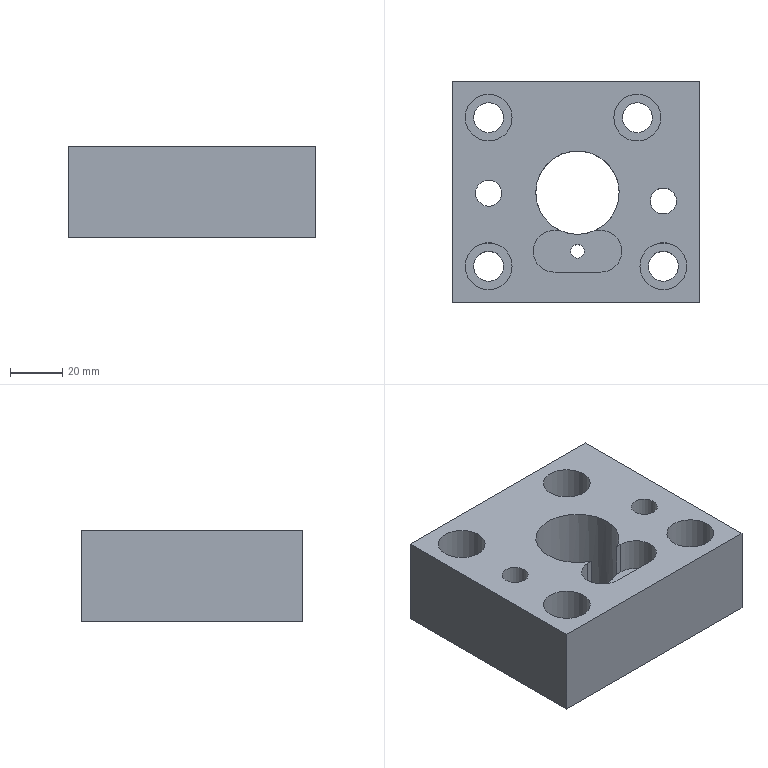Part | STEP file | lll_id4650_x_t | 1 solid | 28 faces | box 95 x 85 x 35 mm | volume 219931 mm3 | plane 14 | cylinder 14 | commonest cylinder face diameters 11.509 x4 18.008 x4 10 x2 16 x2 5.206 x1 32 x1
STEP:
#1=CARTESIAN_POINT('',(888.397,-22.5,-35.));
#2=VERTEX_POINT('',#1);
#3=CARTESIAN_POINT('',(891.,-22.5,-35.));
#4=DIRECTION('',(0.,0.,1.));
#5=DIRECTION('',(-1.,0.,0.));
#6=AXIS2_PLACEMENT_3D('',#3,#4,#5);
#7=CIRCLE('',#6,2.603);
#8=EDGE_CURVE('',#2,#2,#7,.T.);
#9=ORIENTED_EDGE('',*,*,#8,.T.);
#10=EDGE_LOOP('',(#9));
#11=FACE_BOUND('',#10,.T.);
#12=CARTESIAN_POINT('',(875.,0.,-35.));
#13=VERTEX_POINT('',#12);
#14=CARTESIAN_POINT('',(891.,0.,-35.));
#15=DIRECTION('',(0.,0.,1.));
#16=DIRECTION('',(-1.,0.,0.));
#17=AXIS2_PLACEMENT_3D('',#14,#15,#16);
#18=CIRCLE('',#17,16.);
#19=EDGE_CURVE('',#13,#13,#18,.T.);
#20=ORIENTED_EDGE('',*,*,#19,.T.);
#21=EDGE_LOOP('',(#20));
#22=FACE_BOUND('',#21,.T.);
#23=CARTESIAN_POINT('',(842.935,42.75,-35.));
#24=VERTEX_POINT('',#23);
#25=CARTESIAN_POINT('',(842.935,-42.25,-35.));
#26=VERTEX_POINT('',#25);
#27=CARTESIAN_POINT('',(842.935,10.25,-35.));
#28=DIRECTION('',(0.,-1.,0.));
#29=VECTOR('',#28,1.);
#30=LINE('',#27,#29);
#31=EDGE_CURVE('',#24,#26,#30,.T.);
#32=ORIENTED_EDGE('',*,*,#31,.F.);
#33=CARTESIAN_POINT('',(937.935,42.75,-35.));
#34=VERTEX_POINT('',#33);
#35=CARTESIAN_POINT('',(920.435,42.75,-35.));
#36=DIRECTION('',(-1.,0.,0.));
#37=VECTOR('',#36,1.);
#38=LINE('',#35,#37);
#39=EDGE_CURVE('',#34,#24,#38,.T.);
#40=ORIENTED_EDGE('',*,*,#39,.F.);
#41=CARTESIAN_POINT('',(937.935,-42.25,-35.));
#42=VERTEX_POINT('',#41);
#43=CARTESIAN_POINT('',(937.935,10.25,-35.));
#44=DIRECTION('',(0.,1.,0.));
#45=VECTOR('',#44,1.);
#46=LINE('',#43,#45);
#47=EDGE_CURVE('',#42,#34,#46,.T.);
#48=ORIENTED_EDGE('',*,*,#47,.F.);
#49=CARTESIAN_POINT('',(920.435,-42.25,-35.));
#50=DIRECTION('',(1.,0.,0.));
#51=VECTOR('',#50,1.);
#52=LINE('',#49,#51);
#53=EDGE_CURVE('',#26,#42,#52,.T.);
#54=ORIENTED_EDGE('',*,*,#53,.F.);
#55=EDGE_LOOP('',(#32,#40,#48,#54));
#56=FACE_BOUND('',#55,.T.);
#57=CARTESIAN_POINT('',(919.69,28.75,-35.));
#58=VERTEX_POINT('',#57);
#59=CARTESIAN_POINT('',(913.935,28.75,-35.));
#60=DIRECTION('',(0.,0.,-1.));
#61=DIRECTION('',(1.,0.,0.));
#62=AXIS2_PLACEMENT_3D('',#59,#60,#61);
#63=CIRCLE('',#62,5.755);
#64=EDGE_CURVE('',#58,#58,#63,.T.);
#65=ORIENTED_EDGE('',*,*,#64,.F.);
#66=EDGE_LOOP('',(#65));
#67=FACE_BOUND('',#66,.T.);
#68=CARTESIAN_POINT('',(929.69,-28.25,-35.));
#69=VERTEX_POINT('',#68);
#70=CARTESIAN_POINT('',(923.935,-28.25,-35.));
#71=DIRECTION('',(0.,0.,-1.));
#72=DIRECTION('',(1.,0.,0.));
#73=AXIS2_PLACEMENT_3D('',#70,#71,#72);
#74=CIRCLE('',#73,5.755);
#75=EDGE_CURVE('',#69,#69,#74,.T.);
#76=ORIENTED_EDGE('',*,*,#75,.F.);
#77=EDGE_LOOP('',(#76));
#78=FACE_BOUND('',#77,.T.);
#79=CARTESIAN_POINT('',(928.935,-3.25,-35.));
#80=VERTEX_POINT('',#79);
#81=CARTESIAN_POINT('',(923.935,-3.25,-35.));
#82=DIRECTION('',(0.,0.,-1.));
#83=DIRECTION('',(1.,0.,0.));
#84=AXIS2_PLACEMENT_3D('',#81,#82,#83);
#85=CIRCLE('',#84,5.);
#86=EDGE_CURVE('',#80,#80,#85,.T.);
#87=ORIENTED_EDGE('',*,*,#86,.F.);
#88=EDGE_LOOP('',(#87));
#89=FACE_BOUND('',#88,.T.);
#90=CARTESIAN_POINT('',(862.69,-28.25,-35.));
#91=VERTEX_POINT('',#90);
#92=CARTESIAN_POINT('',(856.935,-28.25,-35.));
#93=DIRECTION('',(0.,0.,-1.));
#94=DIRECTION('',(1.,0.,0.));
#95=AXIS2_PLACEMENT_3D('',#92,#93,#94);
#96=CIRCLE('',#95,5.755);
#97=EDGE_CURVE('',#91,#91,#96,.T.);
#98=ORIENTED_EDGE('',*,*,#97,.F.);
#99=EDGE_LOOP('',(#98));
#100=FACE_BOUND('',#99,.T.);
#101=CARTESIAN_POINT('',(862.69,28.75,-35.));
#102=VERTEX_POINT('',#101);
#103=CARTESIAN_POINT('',(856.935,28.75,-35.));
#104=DIRECTION('',(0.,0.,-1.));
#105=DIRECTION('',(1.,0.,0.));
#106=AXIS2_PLACEMENT_3D('',#103,#104,#105);
#107=CIRCLE('',#106,5.755);
#108=EDGE_CURVE('',#102,#102,#107,.T.);
#109=ORIENTED_EDGE('',*,*,#108,.F.);
#110=EDGE_LOOP('',(#109));
#111=FACE_BOUND('',#110,.T.);
#112=CARTESIAN_POINT('',(861.935,-0.25,-35.));
#113=VERTEX_POINT('',#112);
#114=CARTESIAN_POINT('',(856.935,-0.25,-35.));
#115=DIRECTION('',(0.,0.,-1.));
#116=DIRECTION('',(1.,0.,0.));
#117=AXIS2_PLACEMENT_3D('',#114,#115,#116);
#118=CIRCLE('',#117,5.);
#119=EDGE_CURVE('',#113,#113,#118,.T.);
#120=ORIENTED_EDGE('',*,*,#119,.F.);
#121=EDGE_LOOP('',(#120));
#122=FACE_BOUND('',#121,.T.);
#123=CARTESIAN_POINT('',(920.435,25.25,-35.));
#124=DIRECTION('',(0.,0.,-1.));
#125=DIRECTION('',(1.,0.,0.));
#126=AXIS2_PLACEMENT_3D('',#123,#124,#125);
#127=PLANE('',#126);
#128=ADVANCED_FACE('',(#11,#22,#56,#67,#78,#89,#100,#111,#122),#127,.T.);
#129=CARTESIAN_POINT('',(882.,-30.5,0.));
#130=VERTEX_POINT('',#129);
#131=CARTESIAN_POINT('',(900.,-30.5,0.));
#132=VERTEX_POINT('',#131);
#133=CARTESIAN_POINT('',(920.435,-30.5,0.));
#134=DIRECTION('',(1.,0.,0.));
#135=VECTOR('',#134,1.);
#136=LINE('',#133,#135);
#137=EDGE_CURVE('',#130,#132,#136,.T.);
#138=ORIENTED_EDGE('',*,*,#137,.F.);
#139=CARTESIAN_POINT('',(882.,-14.5,0.));
#140=VERTEX_POINT('',#139);
#141=CARTESIAN_POINT('',(882.,-22.5,0.));
#142=DIRECTION('',(0.,0.,1.));
#143=DIRECTION('',(1.,0.,0.));
#144=AXIS2_PLACEMENT_3D('',#141,#142,#143);
#145=CIRCLE('',#144,8.);
#146=EDGE_CURVE('',#140,#130,#145,.T.);
#147=ORIENTED_EDGE('',*,*,#146,.F.);
#148=CARTESIAN_POINT('',(884.236,-14.5,0.));
#149=VERTEX_POINT('',#148);
#150=CARTESIAN_POINT('',(920.435,-14.5,0.));
#151=DIRECTION('',(-1.,0.,0.));
#152=VECTOR('',#151,1.);
#153=LINE('',#150,#152);
#154=EDGE_CURVE('',#149,#140,#153,.T.);
#155=ORIENTED_EDGE('',*,*,#154,.F.);
#156=CARTESIAN_POINT('',(897.764,-14.5,0.));
#157=VERTEX_POINT('',#156);
#158=CARTESIAN_POINT('',(891.,0.,0.));
#159=DIRECTION('',(0.,0.,1.));
#160=DIRECTION('',(-1.,0.,0.));
#161=AXIS2_PLACEMENT_3D('',#158,#159,#160);
#162=CIRCLE('',#161,16.);
#163=EDGE_CURVE('',#157,#149,#162,.T.);
#164=ORIENTED_EDGE('',*,*,#163,.F.);
#165=CARTESIAN_POINT('',(900.,-14.5,0.));
#166=VERTEX_POINT('',#165);
#167=CARTESIAN_POINT('',(920.435,-14.5,0.));
#168=DIRECTION('',(-1.,0.,0.));
#169=VECTOR('',#168,1.);
#170=LINE('',#167,#169);
#171=EDGE_CURVE('',#166,#157,#170,.T.);
#172=ORIENTED_EDGE('',*,*,#171,.F.);
#173=CARTESIAN_POINT('',(900.,-22.5,0.));
#174=DIRECTION('',(0.,0.,-1.));
#175=DIRECTION('',(1.,0.,0.));
#176=AXIS2_PLACEMENT_3D('',#173,#174,#175);
#177=CIRCLE('',#176,8.);
#178=EDGE_CURVE('',#166,#132,#177,.T.);
#179=ORIENTED_EDGE('',*,*,#178,.T.);
#180=EDGE_LOOP('',(#138,#147,#155,#164,#172,#179));
#181=FACE_BOUND('',#180,.T.);
#182=CARTESIAN_POINT('',(851.935,-0.25,0.));
#183=VERTEX_POINT('',#182);
#184=CARTESIAN_POINT('',(856.935,-0.25,0.));
#185=DIRECTION('',(0.,0.,1.));
#186=DIRECTION('',(-1.,0.,0.));
#187=AXIS2_PLACEMENT_3D('',#184,#185,#186);
#188=CIRCLE('',#187,5.);
#189=EDGE_CURVE('',#183,#183,#188,.T.);
#190=ORIENTED_EDGE('',*,*,#189,.F.);
#191=EDGE_LOOP('',(#190));
#192=FACE_BOUND('',#191,.T.);
#193=CARTESIAN_POINT('',(847.931,-28.25,0.));
#194=VERTEX_POINT('',#193);
#195=CARTESIAN_POINT('',(856.935,-28.25,0.));
#196=DIRECTION('',(0.,0.,-1.));
#197=DIRECTION('',(-1.,0.,0.));
#198=AXIS2_PLACEMENT_3D('',#195,#196,#197);
#199=CIRCLE('',#198,9.004);
#200=EDGE_CURVE('',#194,#194,#199,.T.);
#201=ORIENTED_EDGE('',*,*,#200,.T.);
#202=EDGE_LOOP('',(#201));
#203=FACE_BOUND('',#202,.T.);
#204=CARTESIAN_POINT('',(918.935,-3.25,0.));
#205=VERTEX_POINT('',#204);
#206=CARTESIAN_POINT('',(923.935,-3.25,0.));
#207=DIRECTION('',(0.,0.,1.));
#208=DIRECTION('',(-1.,0.,0.));
#209=AXIS2_PLACEMENT_3D('',#206,#207,#208);
#210=CIRCLE('',#209,5.);
#211=EDGE_CURVE('',#205,#205,#210,.T.);
#212=ORIENTED_EDGE('',*,*,#211,.F.);
#213=EDGE_LOOP('',(#212));
#214=FACE_BOUND('',#213,.T.);
#215=CARTESIAN_POINT('',(904.931,28.75,0.));
#216=VERTEX_POINT('',#215);
#217=CARTESIAN_POINT('',(913.935,28.75,0.));
#218=DIRECTION('',(0.,0.,-1.));
#219=DIRECTION('',(-1.,0.,0.));
#220=AXIS2_PLACEMENT_3D('',#217,#218,#219);
#221=CIRCLE('',#220,9.004);
#222=EDGE_CURVE('',#216,#216,#221,.T.);
#223=ORIENTED_EDGE('',*,*,#222,.T.);
#224=EDGE_LOOP('',(#223));
#225=FACE_BOUND('',#224,.T.);
#226=CARTESIAN_POINT('',(842.935,42.75,0.));
#227=VERTEX_POINT('',#226);
#228=CARTESIAN_POINT('',(937.935,42.75,0.));
#229=VERTEX_POINT('',#228);
#230=CARTESIAN_POINT('',(920.435,42.75,0.));
#231=DIRECTION('',(1.,0.,0.));
#232=VECTOR('',#231,1.);
#233=LINE('',#230,#232);
#234=EDGE_CURVE('',#227,#229,#233,.T.);
#235=ORIENTED_EDGE('',*,*,#234,.F.);
#236=CARTESIAN_POINT('',(842.935,-42.25,0.));
#237=VERTEX_POINT('',#236);
#238=CARTESIAN_POINT('',(842.935,10.25,0.));
#239=DIRECTION('',(0.,1.,0.));
#240=VECTOR('',#239,1.);
#241=LINE('',#238,#240);
#242=EDGE_CURVE('',#237,#227,#241,.T.);
#243=ORIENTED_EDGE('',*,*,#242,.F.);
#244=CARTESIAN_POINT('',(937.935,-42.25,0.));
#245=VERTEX_POINT('',#244);
#246=CARTESIAN_POINT('',(920.435,-42.25,0.));
#247=DIRECTION('',(-1.,0.,0.));
#248=VECTOR('',#247,1.);
#249=LINE('',#246,#248);
#250=EDGE_CURVE('',#245,#237,#249,.T.);
#251=ORIENTED_EDGE('',*,*,#250,.F.);
#252=CARTESIAN_POINT('',(937.935,10.25,0.));
#253=DIRECTION('',(0.,-1.,0.));
#254=VECTOR('',#253,1.);
#255=LINE('',#252,#254);
#256=EDGE_CURVE('',#229,#245,#255,.T.);
#257=ORIENTED_EDGE('',*,*,#256,.F.);
#258=EDGE_LOOP('',(#235,#243,#251,#257));
#259=FACE_BOUND('',#258,.T.);
#260=CARTESIAN_POINT('',(914.931,-28.25,0.));
#261=VERTEX_POINT('',#260);
#262=CARTESIAN_POINT('',(923.935,-28.25,0.));
#263=DIRECTION('',(0.,0.,-1.));
#264=DIRECTION('',(-1.,0.,0.));
#265=AXIS2_PLACEMENT_3D('',#262,#263,#264);
#266=CIRCLE('',#265,9.004);
#267=EDGE_CURVE('',#261,#261,#266,.T.);
#268=ORIENTED_EDGE('',*,*,#267,.T.);
#269=EDGE_LOOP('',(#268));
#270=FACE_BOUND('',#269,.T.);
#271=CARTESIAN_POINT('',(847.931,28.75,0.));
#272=VERTEX_POINT('',#271);
#273=CARTESIAN_POINT('',(856.935,28.75,0.));
#274=DIRECTION('',(0.,0.,-1.));
#275=DIRECTION('',(-1.,0.,0.));
#276=AXIS2_PLACEMENT_3D('',#273,#274,#275);
#277=CIRCLE('',#276,9.004);
#278=EDGE_CURVE('',#272,#272,#277,.T.);
#279=ORIENTED_EDGE('',*,*,#278,.T.);
#280=EDGE_LOOP('',(#279));
#281=FACE_BOUND('',#280,.T.);
#282=CARTESIAN_POINT('',(920.435,25.25,0.));
#283=DIRECTION('',(0.,0.,1.));
#284=DIRECTION('',(-1.,0.,0.));
#285=AXIS2_PLACEMENT_3D('',#282,#283,#284);
#286=PLANE('',#285);
#287=ADVANCED_FACE('',(#181,#192,#203,#214,#225,#259,#270,#281),#286,.T.);
#288=CARTESIAN_POINT('',(842.935,42.75,-32.));
#289=DIRECTION('',(0.,0.,1.));
#290=VECTOR('',#289,1.);
#291=LINE('',#288,#290);
#292=EDGE_CURVE('',#24,#227,#291,.T.);
#293=ORIENTED_EDGE('',*,*,#292,.T.);
#294=ORIENTED_EDGE('',*,*,#234,.T.);
#295=CARTESIAN_POINT('',(937.935,42.75,-32.));
#296=DIRECTION('',(0.,0.,1.));
#297=VECTOR('',#296,1.);
#298=LINE('',#295,#297);
#299=EDGE_CURVE('',#34,#229,#298,.T.);
#300=ORIENTED_EDGE('',*,*,#299,.F.);
#301=ORIENTED_EDGE('',*,*,#39,.T.);
#302=EDGE_LOOP('',(#293,#294,#300,#301));
#303=FACE_OUTER_BOUND('',#302,.T.);
#304=CARTESIAN_POINT('',(920.435,42.75,-32.));
#305=DIRECTION('',(0.,1.,0.));
#306=DIRECTION('',(0.,0.,-1.));
#307=AXIS2_PLACEMENT_3D('',#304,#305,#306);
#308=PLANE('',#307);
#309=ADVANCED_FACE('',(#303),#308,.T.);
#310=ORIENTED_EDGE('',*,*,#299,.T.);
#311=ORIENTED_EDGE('',*,*,#256,.T.);
#312=CARTESIAN_POINT('',(937.935,-42.25,-32.));
#313=DIRECTION('',(0.,0.,1.));
#314=VECTOR('',#313,1.);
#315=LINE('',#312,#314);
#316=EDGE_CURVE('',#42,#245,#315,.T.);
#317=ORIENTED_EDGE('',*,*,#316,.F.);
#318=ORIENTED_EDGE('',*,*,#47,.T.);
#319=EDGE_LOOP('',(#310,#311,#317,#318));
#320=FACE_OUTER_BOUND('',#319,.T.);
#321=CARTESIAN_POINT('',(937.935,10.25,-32.));
#322=DIRECTION('',(1.,0.,0.));
#323=DIRECTION('',(0.,0.,1.));
#324=AXIS2_PLACEMENT_3D('',#321,#322,#323);
#325=PLANE('',#324);
#326=ADVANCED_FACE('',(#320),#325,.T.);
#327=ORIENTED_EDGE('',*,*,#316,.T.);
#328=ORIENTED_EDGE('',*,*,#250,.T.);
#329=CARTESIAN_POINT('',(842.935,-42.25,-32.));
#330=DIRECTION('',(0.,0.,1.));
#331=VECTOR('',#330,1.);
#332=LINE('',#329,#331);
#333=EDGE_CURVE('',#26,#237,#332,.T.);
#334=ORIENTED_EDGE('',*,*,#333,.F.);
#335=ORIENTED_EDGE('',*,*,#53,.T.);
#336=EDGE_LOOP('',(#327,#328,#334,#335));
#337=FACE_OUTER_BOUND('',#336,.T.);
#338=CARTESIAN_POINT('',(920.435,-42.25,-32.));
#339=DIRECTION('',(0.,-1.,0.));
#340=DIRECTION('',(0.,0.,1.));
#341=AXIS2_PLACEMENT_3D('',#338,#339,#340);
#342=PLANE('',#341);
#343=ADVANCED_FACE('',(#337),#342,.T.);
#344=ORIENTED_EDGE('',*,*,#31,.T.);
#345=ORIENTED_EDGE('',*,*,#333,.T.);
#346=ORIENTED_EDGE('',*,*,#242,.T.);
#347=ORIENTED_EDGE('',*,*,#292,.F.);
#348=EDGE_LOOP('',(#344,#345,#346,#347));
#349=FACE_OUTER_BOUND('',#348,.T.);
#350=CARTESIAN_POINT('',(842.935,10.25,-32.));
#351=DIRECTION('',(-1.,0.,0.));
#352=DIRECTION('',(0.,0.,-1.));
#353=AXIS2_PLACEMENT_3D('',#350,#351,#352);
#354=PLANE('',#353);
#355=ADVANCED_FACE('',(#349),#354,.T.);
#356=ORIENTED_EDGE('',*,*,#64,.T.);
#357=EDGE_LOOP('',(#356));
#358=FACE_BOUND('',#357,.T.);
#359=CARTESIAN_POINT('',(919.69,28.75,-13.));
#360=VERTEX_POINT('',#359);
#361=CARTESIAN_POINT('',(913.935,28.75,-13.));
#362=DIRECTION('',(0.,0.,-1.));
#363=DIRECTION('',(1.,0.,0.));
#364=AXIS2_PLACEMENT_3D('',#361,#362,#363);
#365=CIRCLE('',#364,5.755);
#366=EDGE_CURVE('',#360,#360,#365,.T.);
#367=ORIENTED_EDGE('',*,*,#366,.F.);
#368=EDGE_LOOP('',(#367));
#369=FACE_BOUND('',#368,.T.);
#370=CARTESIAN_POINT('',(913.935,28.75,2.));
#371=DIRECTION('',(0.,0.,-1.));
#372=DIRECTION('',(-1.,0.,0.));
#373=AXIS2_PLACEMENT_3D('',#370,#371,#372);
#374=CYLINDRICAL_SURFACE('',#373,5.755);
#375=ADVANCED_FACE('',(#358,#369),#374,.F.);
#376=ORIENTED_EDGE('',*,*,#366,.T.);
#377=EDGE_LOOP('',(#376));
#378=FACE_BOUND('',#377,.T.);
#379=CARTESIAN_POINT('',(904.931,28.75,-13.));
#380=VERTEX_POINT('',#379);
#381=CARTESIAN_POINT('',(913.935,28.75,-13.));
#382=DIRECTION('',(0.,0.,-1.));
#383=DIRECTION('',(-1.,0.,0.));
#384=AXIS2_PLACEMENT_3D('',#381,#382,#383);
#385=CIRCLE('',#384,9.004);
#386=EDGE_CURVE('',#380,#380,#385,.T.);
#387=ORIENTED_EDGE('',*,*,#386,.F.);
#388=EDGE_LOOP('',(#387));
#389=FACE_BOUND('',#388,.T.);
#390=CARTESIAN_POINT('',(913.935,28.75,-13.));
#391=DIRECTION('',(0.,0.,-1.));
#392=DIRECTION('',(1.,0.,0.));
#393=AXIS2_PLACEMENT_3D('',#390,#391,#392);
#394=PLANE('',#393);
#395=ADVANCED_FACE('',(#378,#389),#394,.F.);
#396=ORIENTED_EDGE('',*,*,#386,.T.);
#397=EDGE_LOOP('',(#396));
#398=FACE_BOUND('',#397,.T.);
#399=ORIENTED_EDGE('',*,*,#222,.F.);
#400=EDGE_LOOP('',(#399));
#401=FACE_BOUND('',#400,.T.);
#402=CARTESIAN_POINT('',(913.935,28.75,0.));
#403=DIRECTION('',(0.,0.,-1.));
#404=DIRECTION('',(-1.,0.,0.));
#405=AXIS2_PLACEMENT_3D('',#402,#403,#404);
#406=CYLINDRICAL_SURFACE('',#405,9.004);
#407=ADVANCED_FACE('',(#398,#401),#406,.F.);
#408=ORIENTED_EDGE('',*,*,#75,.T.);
#409=EDGE_LOOP('',(#408));
#410=FACE_BOUND('',#409,.T.);
#411=CARTESIAN_POINT('',(929.69,-28.25,-13.));
#412=VERTEX_POINT('',#411);
#413=CARTESIAN_POINT('',(923.935,-28.25,-13.));
#414=DIRECTION('',(0.,0.,-1.));
#415=DIRECTION('',(1.,0.,0.));
#416=AXIS2_PLACEMENT_3D('',#413,#414,#415);
#417=CIRCLE('',#416,5.755);
#418=EDGE_CURVE('',#412,#412,#417,.T.);
#419=ORIENTED_EDGE('',*,*,#418,.F.);
#420=EDGE_LOOP('',(#419));
#421=FACE_BOUND('',#420,.T.);
#422=CARTESIAN_POINT('',(923.935,-28.25,2.));
#423=DIRECTION('',(0.,0.,-1.));
#424=DIRECTION('',(-1.,0.,0.));
#425=AXIS2_PLACEMENT_3D('',#422,#423,#424);
#426=CYLINDRICAL_SURFACE('',#425,5.755);
#427=ADVANCED_FACE('',(#410,#421),#426,.F.);
#428=ORIENTED_EDGE('',*,*,#418,.T.);
#429=EDGE_LOOP('',(#428));
#430=FACE_BOUND('',#429,.T.);
#431=CARTESIAN_POINT('',(914.931,-28.25,-13.));
#432=VERTEX_POINT('',#431);
#433=CARTESIAN_POINT('',(923.935,-28.25,-13.));
#434=DIRECTION('',(0.,0.,-1.));
#435=DIRECTION('',(-1.,0.,0.));
#436=AXIS2_PLACEMENT_3D('',#433,#434,#435);
#437=CIRCLE('',#436,9.004);
#438=EDGE_CURVE('',#432,#432,#437,.T.);
#439=ORIENTED_EDGE('',*,*,#438,.F.);
#440=EDGE_LOOP('',(#439));
#441=FACE_BOUND('',#440,.T.);
#442=CARTESIAN_POINT('',(923.935,-28.25,-13.));
#443=DIRECTION('',(0.,0.,-1.));
#444=DIRECTION('',(1.,0.,0.));
#445=AXIS2_PLACEMENT_3D('',#442,#443,#444);
#446=PLANE('',#445);
#447=ADVANCED_FACE('',(#430,#441),#446,.F.);
#448=ORIENTED_EDGE('',*,*,#438,.T.);
#449=EDGE_LOOP('',(#448));
#450=FACE_BOUND('',#449,.T.);
#451=ORIENTED_EDGE('',*,*,#267,.F.);
#452=EDGE_LOOP('',(#451));
#453=FACE_BOUND('',#452,.T.);
#454=CARTESIAN_POINT('',(923.935,-28.25,0.));
#455=DIRECTION('',(0.,0.,-1.));
#456=DIRECTION('',(-1.,0.,0.));
#457=AXIS2_PLACEMENT_3D('',#454,#455,#456);
#458=CYLINDRICAL_SURFACE('',#457,9.004);
#459=ADVANCED_FACE('',(#450,#453),#458,.F.);
#460=ORIENTED_EDGE('',*,*,#211,.T.);
#461=EDGE_LOOP('',(#460));
#462=FACE_BOUND('',#461,.T.);
#463=ORIENTED_EDGE('',*,*,#86,.T.);
#464=EDGE_LOOP('',(#463));
#465=FACE_BOUND('',#464,.T.);
#466=CARTESIAN_POINT('',(923.935,-3.25,2.));
#467=DIRECTION('',(0.,0.,-1.));
#468=DIRECTION('',(-1.,0.,0.));
#469=AXIS2_PLACEMENT_3D('',#466,#467,#468);
#470=CYLINDRICAL_SURFACE('',#469,5.);
#471=ADVANCED_FACE('',(#462,#465),#470,.F.);
#472=ORIENTED_EDGE('',*,*,#97,.T.);
#473=EDGE_LOOP('',(#472));
#474=FACE_BOUND('',#473,.T.);
#475=CARTESIAN_POINT('',(862.69,-28.25,-13.));
#476=VERTEX_POINT('',#475);
#477=CARTESIAN_POINT('',(856.935,-28.25,-13.));
#478=DIRECTION('',(0.,0.,-1.));
#479=DIRECTION('',(1.,0.,0.));
#480=AXIS2_PLACEMENT_3D('',#477,#478,#479);
#481=CIRCLE('',#480,5.755);
#482=EDGE_CURVE('',#476,#476,#481,.T.);
#483=ORIENTED_EDGE('',*,*,#482,.F.);
#484=EDGE_LOOP('',(#483));
#485=FACE_BOUND('',#484,.T.);
#486=CARTESIAN_POINT('',(856.935,-28.25,2.));
#487=DIRECTION('',(0.,0.,-1.));
#488=DIRECTION('',(-1.,0.,0.));
#489=AXIS2_PLACEMENT_3D('',#486,#487,#488);
#490=CYLINDRICAL_SURFACE('',#489,5.755);
#491=ADVANCED_FACE('',(#474,#485),#490,.F.);
#492=ORIENTED_EDGE('',*,*,#482,.T.);
#493=EDGE_LOOP('',(#492));
#494=FACE_BOUND('',#493,.T.);
#495=CARTESIAN_POINT('',(847.931,-28.25,-13.));
#496=VERTEX_POINT('',#495);
#497=CARTESIAN_POINT('',(856.935,-28.25,-13.));
#498=DIRECTION('',(0.,0.,-1.));
#499=DIRECTION('',(-1.,0.,0.));
#500=AXIS2_PLACEMENT_3D('',#497,#498,#499);
#501=CIRCLE('',#500,9.004);
#502=EDGE_CURVE('',#496,#496,#501,.T.);
#503=ORIENTED_EDGE('',*,*,#502,.F.);
#504=EDGE_LOOP('',(#503));
#505=FACE_BOUND('',#504,.T.);
#506=CARTESIAN_POINT('',(856.935,-28.25,-13.));
#507=DIRECTION('',(0.,0.,-1.));
#508=DIRECTION('',(1.,0.,0.));
#509=AXIS2_PLACEMENT_3D('',#506,#507,#508);
#510=PLANE('',#509);
#511=ADVANCED_FACE('',(#494,#505),#510,.F.);
#512=ORIENTED_EDGE('',*,*,#502,.T.);
#513=EDGE_LOOP('',(#512));
#514=FACE_BOUND('',#513,.T.);
#515=ORIENTED_EDGE('',*,*,#200,.F.);
#516=EDGE_LOOP('',(#515));
#517=FACE_BOUND('',#516,.T.);
#518=CARTESIAN_POINT('',(856.935,-28.25,0.));
#519=DIRECTION('',(0.,0.,-1.));
#520=DIRECTION('',(-1.,0.,0.));
#521=AXIS2_PLACEMENT_3D('',#518,#519,#520);
#522=CYLINDRICAL_SURFACE('',#521,9.004);
#523=ADVANCED_FACE('',(#514,#517),#522,.F.);
#524=ORIENTED_EDGE('',*,*,#108,.T.);
#525=EDGE_LOOP('',(#524));
#526=FACE_BOUND('',#525,.T.);
#527=CARTESIAN_POINT('',(862.69,28.75,-13.));
#528=VERTEX_POINT('',#527);
#529=CARTESIAN_POINT('',(856.935,28.75,-13.));
#530=DIRECTION('',(0.,0.,-1.));
#531=DIRECTION('',(1.,0.,0.));
#532=AXIS2_PLACEMENT_3D('',#529,#530,#531);
#533=CIRCLE('',#532,5.755);
#534=EDGE_CURVE('',#528,#528,#533,.T.);
#535=ORIENTED_EDGE('',*,*,#534,.F.);
#536=EDGE_LOOP('',(#535));
#537=FACE_BOUND('',#536,.T.);
#538=CARTESIAN_POINT('',(856.935,28.75,2.));
#539=DIRECTION('',(0.,0.,-1.));
#540=DIRECTION('',(-1.,0.,0.));
#541=AXIS2_PLACEMENT_3D('',#538,#539,#540);
#542=CYLINDRICAL_SURFACE('',#541,5.755);
#543=ADVANCED_FACE('',(#526,#537),#542,.F.);
#544=ORIENTED_EDGE('',*,*,#534,.T.);
#545=EDGE_LOOP('',(#544));
#546=FACE_BOUND('',#545,.T.);
#547=CARTESIAN_POINT('',(847.931,28.75,-13.));
#548=VERTEX_POINT('',#547);
#549=CARTESIAN_POINT('',(856.935,28.75,-13.));
#550=DIRECTION('',(0.,0.,-1.));
#551=DIRECTION('',(-1.,0.,0.));
#552=AXIS2_PLACEMENT_3D('',#549,#550,#551);
#553=CIRCLE('',#552,9.004);
#554=EDGE_CURVE('',#548,#548,#553,.T.);
#555=ORIENTED_EDGE('',*,*,#554,.F.);
#556=EDGE_LOOP('',(#555));
#557=FACE_BOUND('',#556,.T.);
#558=CARTESIAN_POINT('',(856.935,28.75,-13.));
#559=DIRECTION('',(0.,0.,-1.));
#560=DIRECTION('',(1.,0.,0.));
#561=AXIS2_PLACEMENT_3D('',#558,#559,#560);
#562=PLANE('',#561);
#563=ADVANCED_FACE('',(#546,#557),#562,.F.);
#564=ORIENTED_EDGE('',*,*,#554,.T.);
#565=EDGE_LOOP('',(#564));
#566=FACE_BOUND('',#565,.T.);
#567=ORIENTED_EDGE('',*,*,#278,.F.);
#568=EDGE_LOOP('',(#567));
#569=FACE_BOUND('',#568,.T.);
#570=CARTESIAN_POINT('',(856.935,28.75,0.));
#571=DIRECTION('',(0.,0.,-1.));
#572=DIRECTION('',(-1.,0.,0.));
#573=AXIS2_PLACEMENT_3D('',#570,#571,#572);
#574=CYLINDRICAL_SURFACE('',#573,9.004);
#575=ADVANCED_FACE('',(#566,#569),#574,.F.);
#576=ORIENTED_EDGE('',*,*,#189,.T.);
#577=EDGE_LOOP('',(#576));
#578=FACE_BOUND('',#577,.T.);
#579=ORIENTED_EDGE('',*,*,#119,.T.);
#580=EDGE_LOOP('',(#579));
#581=FACE_BOUND('',#580,.T.);
#582=CARTESIAN_POINT('',(856.935,-0.25,2.));
#583=DIRECTION('',(0.,0.,-1.));
#584=DIRECTION('',(-1.,0.,0.));
#585=AXIS2_PLACEMENT_3D('',#582,#583,#584);
#586=CYLINDRICAL_SURFACE('',#585,5.);
#587=ADVANCED_FACE('',(#578,#581),#586,.F.);
#588=ORIENTED_EDGE('',*,*,#8,.F.);
#589=EDGE_LOOP('',(#588));
#590=FACE_BOUND('',#589,.T.);
#591=CARTESIAN_POINT('',(893.603,-22.5,-13.));
#592=VERTEX_POINT('',#591);
#593=CARTESIAN_POINT('',(891.,-22.5,-13.));
#594=DIRECTION('',(0.,0.,-1.));
#595=DIRECTION('',(1.,0.,0.));
#596=AXIS2_PLACEMENT_3D('',#593,#594,#595);
#597=CIRCLE('',#596,2.603);
#598=EDGE_CURVE('',#592,#592,#597,.T.);
#599=ORIENTED_EDGE('',*,*,#598,.F.);
#600=EDGE_LOOP('',(#599));
#601=FACE_BOUND('',#600,.T.);
#602=CARTESIAN_POINT('',(891.,-22.5,-13.));
#603=DIRECTION('',(0.,0.,-1.));
#604=DIRECTION('',(1.,0.,0.));
#605=AXIS2_PLACEMENT_3D('',#602,#603,#604);
#606=CYLINDRICAL_SURFACE('',#605,2.603);
#607=ADVANCED_FACE('',(#590,#601),#606,.F.);
#608=CARTESIAN_POINT('',(882.,-14.5,-13.));
#609=VERTEX_POINT('',#608);
#610=CARTESIAN_POINT('',(882.,-14.5,-1.));
#611=DIRECTION('',(0.,0.,-1.));
#612=VECTOR('',#611,1.);
#613=LINE('',#610,#612);
#614=EDGE_CURVE('',#140,#609,#613,.T.);
#615=ORIENTED_EDGE('',*,*,#614,.T.);
#616=CARTESIAN_POINT('',(884.236,-14.5,-13.));
#617=VERTEX_POINT('',#616);
#618=CARTESIAN_POINT('',(882.,-14.5,-13.));
#619=DIRECTION('',(-1.,0.,0.));
#620=VECTOR('',#619,1.);
#621=LINE('',#618,#620);
#622=EDGE_CURVE('',#617,#609,#621,.T.);
#623=ORIENTED_EDGE('',*,*,#622,.F.);
#624=CARTESIAN_POINT('',(884.236,-14.5,-15.));
#625=DIRECTION('',(0.,0.,1.));
#626=VECTOR('',#625,1.);
#627=LINE('',#624,#626);
#628=EDGE_CURVE('',#617,#149,#627,.T.);
#629=ORIENTED_EDGE('',*,*,#628,.T.);
#630=ORIENTED_EDGE('',*,*,#154,.T.);
#631=EDGE_LOOP('',(#615,#623,#629,#630));
#632=FACE_OUTER_BOUND('',#631,.T.);
#633=CARTESIAN_POINT('',(454.,-14.5,0.));
#634=DIRECTION('',(0.,-1.,0.));
#635=DIRECTION('',(0.,0.,-1.));
#636=AXIS2_PLACEMENT_3D('',#633,#634,#635);
#637=PLANE('',#636);
#638=ADVANCED_FACE('',(#632),#637,.T.);
#639=ORIENTED_EDGE('',*,*,#178,.F.);
#640=CARTESIAN_POINT('',(900.,-14.5,-13.));
#641=VERTEX_POINT('',#640);
#642=CARTESIAN_POINT('',(900.,-14.5,-7.));
#643=DIRECTION('',(0.,0.,1.));
#644=VECTOR('',#643,1.);
#645=LINE('',#642,#644);
#646=EDGE_CURVE('',#641,#166,#645,.T.);
#647=ORIENTED_EDGE('',*,*,#646,.F.);
#648=CARTESIAN_POINT('',(900.,-30.5,-13.));
#649=VERTEX_POINT('',#648);
#650=CARTESIAN_POINT('',(900.,-22.5,-13.));
#651=DIRECTION('',(0.,0.,-1.));
#652=DIRECTION('',(1.,0.,0.));
#653=AXIS2_PLACEMENT_3D('',#650,#651,#652);
#654=CIRCLE('',#653,8.);
#655=EDGE_CURVE('',#641,#649,#654,.T.);
#656=ORIENTED_EDGE('',*,*,#655,.T.);
#657=CARTESIAN_POINT('',(900.,-30.5,-1.));
#658=DIRECTION('',(0.,0.,1.));
#659=VECTOR('',#658,1.);
#660=LINE('',#657,#659);
#661=EDGE_CURVE('',#649,#132,#660,.T.);
#662=ORIENTED_EDGE('',*,*,#661,.T.);
#663=EDGE_LOOP('',(#639,#647,#656,#662));
#664=FACE_OUTER_BOUND('',#663,.T.);
#665=CARTESIAN_POINT('',(900.,-22.5,-1.));
#666=DIRECTION('',(0.,0.,-1.));
#667=DIRECTION('',(1.,0.,0.));
#668=AXIS2_PLACEMENT_3D('',#665,#666,#667);
#669=CYLINDRICAL_SURFACE('',#668,8.);
#670=ADVANCED_FACE('',(#664),#669,.F.);
#671=ORIENTED_EDGE('',*,*,#137,.T.);
#672=ORIENTED_EDGE('',*,*,#661,.F.);
#673=CARTESIAN_POINT('',(882.,-30.5,-13.));
#674=VERTEX_POINT('',#673);
#675=CARTESIAN_POINT('',(882.,-30.5,-13.));
#676=DIRECTION('',(-1.,0.,0.));
#677=VECTOR('',#676,1.);
#678=LINE('',#675,#677);
#679=EDGE_CURVE('',#649,#674,#678,.T.);
#680=ORIENTED_EDGE('',*,*,#679,.T.);
#681=CARTESIAN_POINT('',(882.,-30.5,-1.));
#682=DIRECTION('',(0.,0.,-1.));
#683=VECTOR('',#682,1.);
#684=LINE('',#681,#683);
#685=EDGE_CURVE('',#130,#674,#684,.T.);
#686=ORIENTED_EDGE('',*,*,#685,.F.);
#687=EDGE_LOOP('',(#671,#672,#680,#686));
#688=FACE_OUTER_BOUND('',#687,.T.);
#689=CARTESIAN_POINT('',(454.,-30.5,0.));
#690=DIRECTION('',(0.,-1.,0.));
#691=DIRECTION('',(0.,0.,-1.));
#692=AXIS2_PLACEMENT_3D('',#689,#690,#691);
#693=PLANE('',#692);
#694=ADVANCED_FACE('',(#688),#693,.F.);
#695=CARTESIAN_POINT('',(897.764,-14.5,-13.));
#696=VERTEX_POINT('',#695);
#697=CARTESIAN_POINT('',(891.,0.,-13.));
#698=DIRECTION('',(0.,0.,-1.));
#699=DIRECTION('',(1.,0.,0.));
#700=AXIS2_PLACEMENT_3D('',#697,#698,#699);
#701=CIRCLE('',#700,16.);
#702=EDGE_CURVE('',#696,#617,#701,.T.);
#703=ORIENTED_EDGE('',*,*,#702,.T.);
#704=ORIENTED_EDGE('',*,*,#622,.T.);
#705=CARTESIAN_POINT('',(882.,-22.5,-13.));
#706=DIRECTION('',(0.,0.,-1.));
#707=DIRECTION('',(1.,0.,0.));
#708=AXIS2_PLACEMENT_3D('',#705,#706,#707);
#709=CIRCLE('',#708,8.);
#710=EDGE_CURVE('',#674,#609,#709,.T.);
#711=ORIENTED_EDGE('',*,*,#710,.F.);
#712=ORIENTED_EDGE('',*,*,#679,.F.);
#713=ORIENTED_EDGE('',*,*,#655,.F.);
#714=CARTESIAN_POINT('',(882.,-14.5,-13.));
#715=DIRECTION('',(-1.,0.,0.));
#716=VECTOR('',#715,1.);
#717=LINE('',#714,#716);
#718=EDGE_CURVE('',#641,#696,#717,.T.);
#719=ORIENTED_EDGE('',*,*,#718,.T.);
#720=EDGE_LOOP('',(#703,#704,#711,#712,#713,#719));
#721=FACE_BOUND('',#720,.T.);
#722=ORIENTED_EDGE('',*,*,#598,.T.);
#723=EDGE_LOOP('',(#722));
#724=FACE_BOUND('',#723,.T.);
#725=CARTESIAN_POINT('',(882.,-22.5,-13.));
#726=DIRECTION('',(0.,0.,1.));
#727=DIRECTION('',(1.,0.,0.));
#728=AXIS2_PLACEMENT_3D('',#725,#726,#727);
#729=PLANE('',#728);
#730=ADVANCED_FACE('',(#721,#724),#729,.T.);
#731=ORIENTED_EDGE('',*,*,#146,.T.);
#732=ORIENTED_EDGE('',*,*,#685,.T.);
#733=ORIENTED_EDGE('',*,*,#710,.T.);
#734=ORIENTED_EDGE('',*,*,#614,.F.);
#735=EDGE_LOOP('',(#731,#732,#733,#734));
#736=FACE_OUTER_BOUND('',#735,.T.);
#737=CARTESIAN_POINT('',(882.,-22.5,-1.));
#738=DIRECTION('',(0.,0.,-1.));
#739=DIRECTION('',(1.,0.,0.));
#740=AXIS2_PLACEMENT_3D('',#737,#738,#739);
#741=CYLINDRICAL_SURFACE('',#740,8.);
#742=ADVANCED_FACE('',(#736),#741,.F.);
#743=CARTESIAN_POINT('',(897.764,-14.5,-15.));
#744=DIRECTION('',(0.,0.,-1.));
#745=VECTOR('',#744,1.);
#746=LINE('',#743,#745);
#747=EDGE_CURVE('',#157,#696,#746,.T.);
#748=ORIENTED_EDGE('',*,*,#747,.T.);
#749=ORIENTED_EDGE('',*,*,#718,.F.);
#750=ORIENTED_EDGE('',*,*,#646,.T.);
#751=ORIENTED_EDGE('',*,*,#171,.T.);
#752=EDGE_LOOP('',(#748,#749,#750,#751));
#753=FACE_OUTER_BOUND('',#752,.T.);
#754=CARTESIAN_POINT('',(454.,-14.5,0.));
#755=DIRECTION('',(0.,-1.,0.));
#756=DIRECTION('',(0.,0.,-1.));
#757=AXIS2_PLACEMENT_3D('',#754,#755,#756);
#758=PLANE('',#757);
#759=ADVANCED_FACE('',(#753),#758,.T.);
#760=ORIENTED_EDGE('',*,*,#628,.F.);
#761=ORIENTED_EDGE('',*,*,#702,.F.);
#762=ORIENTED_EDGE('',*,*,#747,.F.);
#763=ORIENTED_EDGE('',*,*,#163,.T.);
#764=EDGE_LOOP('',(#760,#761,#762,#763));
#765=FACE_BOUND('',#764,.T.);
#766=ORIENTED_EDGE('',*,*,#19,.F.);
#767=EDGE_LOOP('',(#766));
#768=FACE_BOUND('',#767,.T.);
#769=CARTESIAN_POINT('',(891.,0.,-15.));
#770=DIRECTION('',(0.,0.,-1.));
#771=DIRECTION('',(0.,1.,0.));
#772=AXIS2_PLACEMENT_3D('',#769,#770,#771);
#773=CYLINDRICAL_SURFACE('',#772,16.);
#774=ADVANCED_FACE('',(#765,#768),#773,.F.);
#775=CLOSED_SHELL('',(#128,#287,#309,#326,#343,#355,#375,#395,#407,#427,#447,#459,#471,#491,#511,#523,#543,#563,#575,#587,#607,#638,#670,#694,#730,#742,#759,#774));
#776=MANIFOLD_SOLID_BREP('',#775);
#777=(LENGTH_UNIT()NAMED_UNIT(*)SI_UNIT(.MILLI.,.METRE.));
#778=UNCERTAINTY_MEASURE_WITH_UNIT(LENGTH_MEASURE(0.00002),#777,'','');
#779=(NAMED_UNIT(*)PLANE_ANGLE_UNIT()SI_UNIT($,.RADIAN.));
#780=PLANE_ANGLE_MEASURE_WITH_UNIT(PLANE_ANGLE_MEASURE(0.01745),#779);
#781=DIMENSIONAL_EXPONENTS(0.,0.,0.,0.,0.,0.,0.);
#782=(CONVERSION_BASED_UNIT('DEGREE',#780)NAMED_UNIT(#781)PLANE_ANGLE_UNIT());
#783=(NAMED_UNIT(*)SI_UNIT($,.STERADIAN.)SOLID_ANGLE_UNIT());
#784=(GEOMETRIC_REPRESENTATION_CONTEXT(3)GLOBAL_UNCERTAINTY_ASSIGNED_CONTEXT((#778))GLOBAL_UNIT_ASSIGNED_CONTEXT((#777,#782,#783))REPRESENTATION_CONTEXT('',''));
#785=ADVANCED_BREP_SHAPE_REPRESENTATION('',(#776),#784);